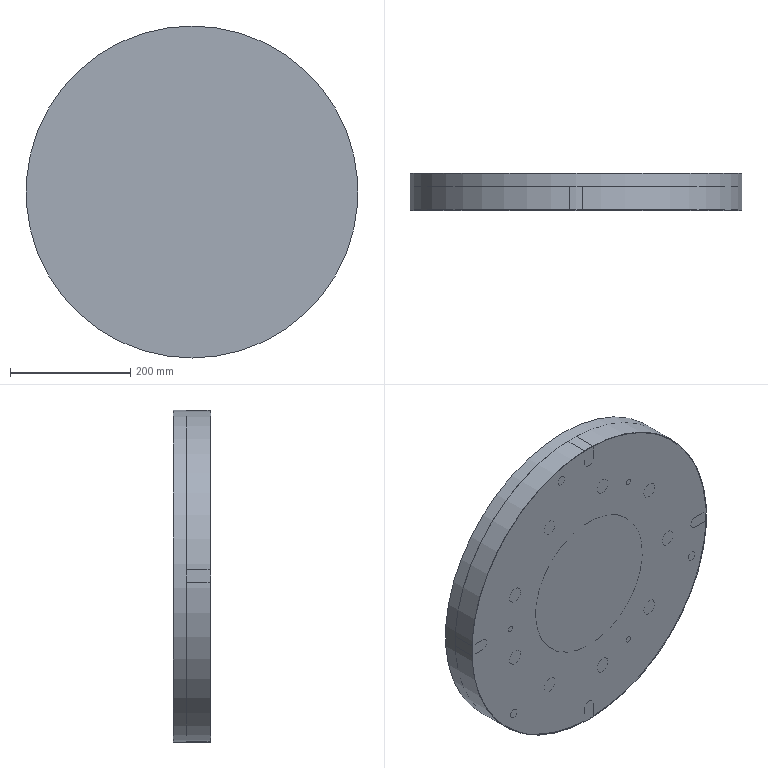Part | 4 solids | 228 faces | box 552 x 62 x 552 mm | volume 46180059 mm3 | plane 144 | cylinder 84 | commonest cylinder face diameters 9 x18 25 x18 390 x10 26 x9 550 x5 20 x4